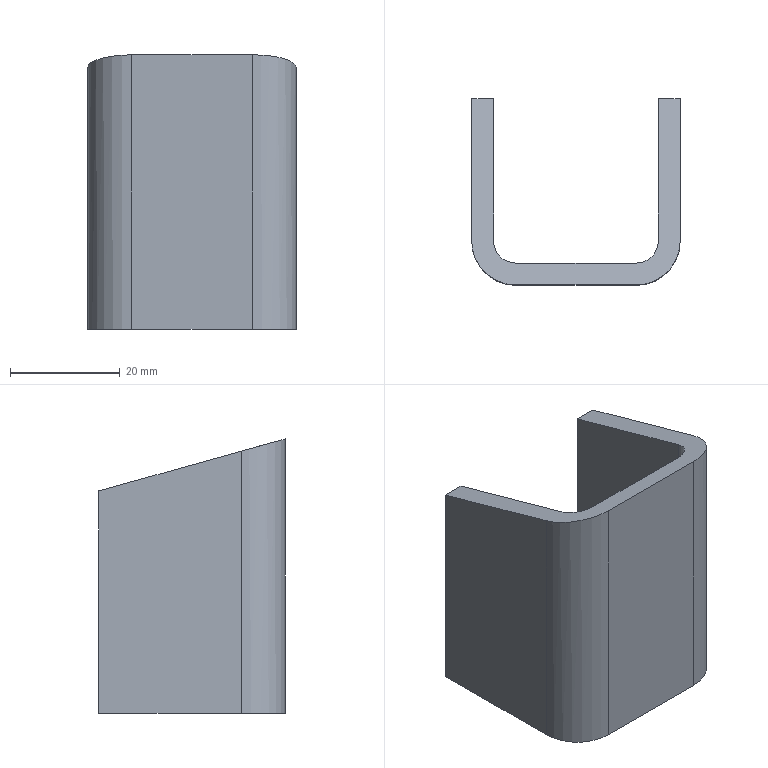Part | STEP file | 18-Reinforcing bent plate 2 | 1 solid | 18 faces | box 38 x 34 x 50 mm | volume 17215 mm3 | plane 14 | cylinder 4 | commonest cylinder face diameters 8 x2 16 x2
STEP:
#1=CARTESIAN_POINT('',(0.,0.,0.));
#2=DIRECTION('',(0.,0.,1.));
#3=DIRECTION('',(1.,0.,0.));
#4=AXIS2_PLACEMENT_3D('',#1,#2,#3);
#5=CARTESIAN_POINT('',(8.,-34.,0.));
#6=VERTEX_POINT('',#5);
#7=CARTESIAN_POINT('',(8.,-30.,0.));
#8=VERTEX_POINT('',#7);
#9=CARTESIAN_POINT('',(8.,-34.,0.));
#10=DIRECTION('',(0.,1.,0.));
#11=VECTOR('',#10,1.);
#12=LINE('',#9,#11);
#13=CARTESIAN_POINT('',(8.,-34.,0.));
#14=DIRECTION('',(0.,0.,-1.));
#15=DIRECTION('',(-1.,0.,0.));
#16=AXIS2_PLACEMENT_3D('',#13,#14,#15);
#17=PLANE('',#16);
#18=CARTESIAN_POINT('',(0.,0.));
#19=DIRECTION('',(0.,1.));
#20=VECTOR('',#19,1.);
#21=LINE('',#18,#20);
#22=(GEOMETRIC_REPRESENTATION_CONTEXT(2)PARAMETRIC_REPRESENTATION_CONTEXT()REPRESENTATION_CONTEXT('',''));
#23=DEFINITIONAL_REPRESENTATION('',(#21),#22);
#24=PCURVE('',#17,#23);
#25=CARTESIAN_POINT('',(4.,-26.,0.));
#26=DIRECTION('',(0.,0.,-1.));
#27=DIRECTION('',(-1.,0.,0.));
#28=AXIS2_PLACEMENT_3D('',#25,#26,#27);
#29=PLANE('',#28);
#30=CARTESIAN_POINT('',(-4.,-8.));
#31=DIRECTION('',(0.,1.));
#32=VECTOR('',#31,1.);
#33=LINE('',#30,#32);
#34=(GEOMETRIC_REPRESENTATION_CONTEXT(2)PARAMETRIC_REPRESENTATION_CONTEXT()REPRESENTATION_CONTEXT('',''));
#35=DEFINITIONAL_REPRESENTATION('',(#33),#34);
#36=PCURVE('',#29,#35);
#37=SURFACE_CURVE('',#12,(#24,#36),.PCURVE_S1.);
#38=EDGE_CURVE('',#6,#8,#37,.T.);
#39=ORIENTED_EDGE('',*,*,#38,.F.);
#40=CARTESIAN_POINT('',(0.,-26.,0.));
#41=VERTEX_POINT('',#40);
#42=CARTESIAN_POINT('',(8.,-26.,0.));
#43=DIRECTION('',(0.,0.,1.));
#44=DIRECTION('',(-1.,0.,0.));
#45=AXIS2_PLACEMENT_3D('',#42,#43,#44);
#46=CIRCLE('',#45,8.);
#47=CARTESIAN_POINT('',(8.,8.));
#48=CARTESIAN_POINT('',(8.,-5.856));
#49=CARTESIAN_POINT('',(-4.,1.072));
#50=CARTESIAN_POINT('',(-16.,8.));
#51=CARTESIAN_POINT('',(-4.,14.928));
#52=CARTESIAN_POINT('',(8.,21.856));
#53=CARTESIAN_POINT('',(8.,8.));
#54=(BOUNDED_CURVE()B_SPLINE_CURVE(2,(#47,#48,#49,#50,#51,#52,#53),.UNSPECIFIED.,.T.,.F.)B_SPLINE_CURVE_WITH_KNOTS((1,2,2,2,2,1),(-2.094,0.,2.094,4.189,6.283,8.378),.UNSPECIFIED.)CURVE()GEOMETRIC_REPRESENTATION_ITEM()RATIONAL_B_SPLINE_CURVE((1.,0.5,1.,0.5,1.,0.5,1.))REPRESENTATION_ITEM(''));
#55=(GEOMETRIC_REPRESENTATION_CONTEXT(2)PARAMETRIC_REPRESENTATION_CONTEXT()REPRESENTATION_CONTEXT('',''));
#56=DEFINITIONAL_REPRESENTATION('',(#54),#55);
#57=PCURVE('',#17,#56);
#58=CARTESIAN_POINT('',(8.,-26.,50.));
#59=DIRECTION('',(0.,0.,-1.));
#60=DIRECTION('',(-1.,0.,0.));
#61=AXIS2_PLACEMENT_3D('',#58,#59,#60);
#62=CYLINDRICAL_SURFACE('',#61,8.);
#63=CARTESIAN_POINT('',(6.283,50.));
#64=DIRECTION('',(-1.,0.));
#65=VECTOR('',#64,1.);
#66=LINE('',#63,#65);
#67=(GEOMETRIC_REPRESENTATION_CONTEXT(2)PARAMETRIC_REPRESENTATION_CONTEXT()REPRESENTATION_CONTEXT('',''));
#68=DEFINITIONAL_REPRESENTATION('',(#66),#67);
#69=PCURVE('',#62,#68);
#70=SURFACE_CURVE('',#46,(#57,#69),.PCURVE_S1.);
#71=EDGE_CURVE('',#41,#6,#70,.T.);
#72=ORIENTED_EDGE('',*,*,#71,.F.);
#73=CARTESIAN_POINT('',(4.,-26.,0.));
#74=VERTEX_POINT('',#73);
#75=CARTESIAN_POINT('',(4.,-26.,0.));
#76=DIRECTION('',(-1.,0.,0.));
#77=VECTOR('',#76,1.);
#78=LINE('',#75,#77);
#79=CARTESIAN_POINT('',(4.,8.));
#80=DIRECTION('',(1.,0.));
#81=VECTOR('',#80,1.);
#82=LINE('',#79,#81);
#83=(GEOMETRIC_REPRESENTATION_CONTEXT(2)PARAMETRIC_REPRESENTATION_CONTEXT()REPRESENTATION_CONTEXT('',''));
#84=DEFINITIONAL_REPRESENTATION('',(#82),#83);
#85=PCURVE('',#17,#84);
#86=CARTESIAN_POINT('',(30.,-26.,0.));
#87=DIRECTION('',(0.,0.,1.));
#88=DIRECTION('',(1.,0.,0.));
#89=AXIS2_PLACEMENT_3D('',#86,#87,#88);
#90=PLANE('',#89);
#91=CARTESIAN_POINT('',(-26.,0.));
#92=DIRECTION('',(-1.,0.));
#93=VECTOR('',#92,1.);
#94=LINE('',#91,#93);
#95=(GEOMETRIC_REPRESENTATION_CONTEXT(2)PARAMETRIC_REPRESENTATION_CONTEXT()REPRESENTATION_CONTEXT('',''));
#96=DEFINITIONAL_REPRESENTATION('',(#94),#95);
#97=PCURVE('',#90,#96);
#98=SURFACE_CURVE('',#78,(#85,#97),.PCURVE_S1.);
#99=EDGE_CURVE('',#74,#41,#98,.T.);
#100=ORIENTED_EDGE('',*,*,#99,.F.);
#101=CARTESIAN_POINT('',(8.,-26.,0.));
#102=DIRECTION('',(0.,0.,1.));
#103=DIRECTION('',(1.,0.,0.));
#104=AXIS2_PLACEMENT_3D('',#101,#102,#103);
#105=CIRCLE('',#104,4.);
#106=CARTESIAN_POINT('',(-4.,8.));
#107=CARTESIAN_POINT('',(-4.,14.928));
#108=CARTESIAN_POINT('',(2.,11.464));
#109=CARTESIAN_POINT('',(8.,8.));
#110=CARTESIAN_POINT('',(2.,4.536));
#111=CARTESIAN_POINT('',(-4.,1.072));
#112=CARTESIAN_POINT('',(-4.,8.));
#113=(BOUNDED_CURVE()B_SPLINE_CURVE(2,(#106,#107,#108,#109,#110,#111,#112),.UNSPECIFIED.,.T.,.F.)B_SPLINE_CURVE_WITH_KNOTS((1,2,2,2,2,1),(-2.094,0.,2.094,4.189,6.283,8.378),.UNSPECIFIED.)CURVE()GEOMETRIC_REPRESENTATION_ITEM()RATIONAL_B_SPLINE_CURVE((1.,0.5,1.,0.5,1.,0.5,1.))REPRESENTATION_ITEM(''));
#114=(GEOMETRIC_REPRESENTATION_CONTEXT(2)PARAMETRIC_REPRESENTATION_CONTEXT()REPRESENTATION_CONTEXT('',''));
#115=DEFINITIONAL_REPRESENTATION('',(#113),#114);
#116=PCURVE('',#17,#115);
#117=CARTESIAN_POINT('',(8.,-26.,50.));
#118=DIRECTION('',(0.,0.,-1.));
#119=DIRECTION('',(-1.,0.,0.));
#120=AXIS2_PLACEMENT_3D('',#117,#118,#119);
#121=CYLINDRICAL_SURFACE('',#120,4.);
#122=CARTESIAN_POINT('',(9.425,50.));
#123=DIRECTION('',(-1.,0.));
#124=VECTOR('',#123,1.);
#125=LINE('',#122,#124);
#126=(GEOMETRIC_REPRESENTATION_CONTEXT(2)PARAMETRIC_REPRESENTATION_CONTEXT()REPRESENTATION_CONTEXT('',''));
#127=DEFINITIONAL_REPRESENTATION('',(#125),#126);
#128=PCURVE('',#121,#127);
#129=SURFACE_CURVE('',#105,(#116,#128),.PCURVE_S1.);
#130=EDGE_CURVE('',#74,#8,#129,.T.);
#131=ORIENTED_EDGE('',*,*,#130,.T.);
#132=EDGE_LOOP('',(#39,#72,#100,#131));
#133=FACE_BOUND('',#132,.T.);
#134=ADVANCED_FACE('',(#133),#17,.T.);
#135=CARTESIAN_POINT('',(30.,-34.,0.));
#136=VERTEX_POINT('',#135);
#137=CARTESIAN_POINT('',(0.,-34.,0.));
#138=DIRECTION('',(1.,0.,0.));
#139=VECTOR('',#138,1.);
#140=LINE('',#137,#139);
#141=CARTESIAN_POINT('',(4.,-8.));
#142=DIRECTION('',(-1.,0.));
#143=VECTOR('',#142,1.);
#144=LINE('',#141,#143);
#145=(GEOMETRIC_REPRESENTATION_CONTEXT(2)PARAMETRIC_REPRESENTATION_CONTEXT()REPRESENTATION_CONTEXT('',''));
#146=DEFINITIONAL_REPRESENTATION('',(#144),#145);
#147=PCURVE('',#29,#146);
#148=CARTESIAN_POINT('',(0.,-34.,50.));
#149=DIRECTION('',(0.,1.,0.));
#150=DIRECTION('',(0.,0.,1.));
#151=AXIS2_PLACEMENT_3D('',#148,#149,#150);
#152=PLANE('',#151);
#153=CARTESIAN_POINT('',(-50.,0.));
#154=DIRECTION('',(0.,1.));
#155=VECTOR('',#154,1.);
#156=LINE('',#153,#155);
#157=(GEOMETRIC_REPRESENTATION_CONTEXT(2)PARAMETRIC_REPRESENTATION_CONTEXT()REPRESENTATION_CONTEXT('',''));
#158=DEFINITIONAL_REPRESENTATION('',(#156),#157);
#159=PCURVE('',#152,#158);
#160=SURFACE_CURVE('',#140,(#147,#159),.PCURVE_S1.);
#161=EDGE_CURVE('',#6,#136,#160,.T.);
#162=ORIENTED_EDGE('',*,*,#161,.F.);
#163=ORIENTED_EDGE('',*,*,#38,.T.);
#164=CARTESIAN_POINT('',(30.,-30.,0.));
#165=VERTEX_POINT('',#164);
#166=CARTESIAN_POINT('',(0.,-30.,0.));
#167=DIRECTION('',(1.,0.,0.));
#168=VECTOR('',#167,1.);
#169=LINE('',#166,#168);
#170=CARTESIAN_POINT('',(4.,-4.));
#171=DIRECTION('',(-1.,0.));
#172=VECTOR('',#171,1.);
#173=LINE('',#170,#172);
#174=(GEOMETRIC_REPRESENTATION_CONTEXT(2)PARAMETRIC_REPRESENTATION_CONTEXT()REPRESENTATION_CONTEXT('',''));
#175=DEFINITIONAL_REPRESENTATION('',(#173),#174);
#176=PCURVE('',#29,#175);
#177=CARTESIAN_POINT('',(0.,-30.,50.));
#178=DIRECTION('',(0.,1.,0.));
#179=DIRECTION('',(0.,0.,1.));
#180=AXIS2_PLACEMENT_3D('',#177,#178,#179);
#181=PLANE('',#180);
#182=CARTESIAN_POINT('',(-50.,0.));
#183=DIRECTION('',(0.,1.));
#184=VECTOR('',#183,1.);
#185=LINE('',#182,#184);
#186=(GEOMETRIC_REPRESENTATION_CONTEXT(2)PARAMETRIC_REPRESENTATION_CONTEXT()REPRESENTATION_CONTEXT('',''));
#187=DEFINITIONAL_REPRESENTATION('',(#185),#186);
#188=PCURVE('',#181,#187);
#189=SURFACE_CURVE('',#169,(#176,#188),.PCURVE_S1.);
#190=EDGE_CURVE('',#8,#165,#189,.T.);
#191=ORIENTED_EDGE('',*,*,#190,.T.);
#192=CARTESIAN_POINT('',(30.,-30.,0.));
#193=DIRECTION('',(0.,-1.,0.));
#194=VECTOR('',#193,1.);
#195=LINE('',#192,#194);
#196=CARTESIAN_POINT('',(-26.,-4.));
#197=DIRECTION('',(0.,-1.));
#198=VECTOR('',#197,1.);
#199=LINE('',#196,#198);
#200=(GEOMETRIC_REPRESENTATION_CONTEXT(2)PARAMETRIC_REPRESENTATION_CONTEXT()REPRESENTATION_CONTEXT('',''));
#201=DEFINITIONAL_REPRESENTATION('',(#199),#200);
#202=PCURVE('',#29,#201);
#203=CARTESIAN_POINT('',(38.,-26.,0.));
#204=DIRECTION('',(0.,0.,-1.));
#205=DIRECTION('',(-1.,0.,0.));
#206=AXIS2_PLACEMENT_3D('',#203,#204,#205);
#207=PLANE('',#206);
#208=CARTESIAN_POINT('',(8.,-4.));
#209=DIRECTION('',(0.,-1.));
#210=VECTOR('',#209,1.);
#211=LINE('',#208,#210);
#212=(GEOMETRIC_REPRESENTATION_CONTEXT(2)PARAMETRIC_REPRESENTATION_CONTEXT()REPRESENTATION_CONTEXT('',''));
#213=DEFINITIONAL_REPRESENTATION('',(#211),#212);
#214=PCURVE('',#207,#213);
#215=SURFACE_CURVE('',#195,(#202,#214),.PCURVE_S1.);
#216=EDGE_CURVE('',#165,#136,#215,.T.);
#217=ORIENTED_EDGE('',*,*,#216,.T.);
#218=EDGE_LOOP('',(#162,#163,#191,#217));
#219=FACE_BOUND('',#218,.T.);
#220=ADVANCED_FACE('',(#219),#29,.T.);
#221=CARTESIAN_POINT('',(38.,-26.,0.));
#222=VERTEX_POINT('',#221);
#223=CARTESIAN_POINT('',(34.,-26.,0.));
#224=VERTEX_POINT('',#223);
#225=CARTESIAN_POINT('',(38.,-26.,0.));
#226=DIRECTION('',(-1.,0.,0.));
#227=VECTOR('',#226,1.);
#228=LINE('',#225,#227);
#229=CARTESIAN_POINT('',(0.,0.));
#230=DIRECTION('',(1.,0.));
#231=VECTOR('',#230,1.);
#232=LINE('',#229,#231);
#233=(GEOMETRIC_REPRESENTATION_CONTEXT(2)PARAMETRIC_REPRESENTATION_CONTEXT()REPRESENTATION_CONTEXT('',''));
#234=DEFINITIONAL_REPRESENTATION('',(#232),#233);
#235=PCURVE('',#207,#234);
#236=CARTESIAN_POINT('',(30.,-30.,0.));
#237=DIRECTION('',(0.,0.,-1.));
#238=DIRECTION('',(-1.,0.,0.));
#239=AXIS2_PLACEMENT_3D('',#236,#237,#238);
#240=PLANE('',#239);
#241=CARTESIAN_POINT('',(-8.,4.));
#242=DIRECTION('',(1.,0.));
#243=VECTOR('',#242,1.);
#244=LINE('',#241,#243);
#245=(GEOMETRIC_REPRESENTATION_CONTEXT(2)PARAMETRIC_REPRESENTATION_CONTEXT()REPRESENTATION_CONTEXT('',''));
#246=DEFINITIONAL_REPRESENTATION('',(#244),#245);
#247=PCURVE('',#240,#246);
#248=SURFACE_CURVE('',#228,(#235,#247),.PCURVE_S1.);
#249=EDGE_CURVE('',#222,#224,#248,.T.);
#250=ORIENTED_EDGE('',*,*,#249,.F.);
#251=CARTESIAN_POINT('',(30.,-26.,0.));
#252=DIRECTION('',(0.,0.,1.));
#253=DIRECTION('',(-1.,0.,0.));
#254=AXIS2_PLACEMENT_3D('',#251,#252,#253);
#255=CIRCLE('',#254,8.);
#256=CARTESIAN_POINT('',(16.,0.));
#257=CARTESIAN_POINT('',(16.,-13.856));
#258=CARTESIAN_POINT('',(4.,-6.928));
#259=CARTESIAN_POINT('',(-8.,0.));
#260=CARTESIAN_POINT('',(4.,6.928));
#261=CARTESIAN_POINT('',(16.,13.856));
#262=CARTESIAN_POINT('',(16.,0.));
#263=(BOUNDED_CURVE()B_SPLINE_CURVE(2,(#256,#257,#258,#259,#260,#261,#262),.UNSPECIFIED.,.T.,.F.)B_SPLINE_CURVE_WITH_KNOTS((1,2,2,2,2,1),(-2.094,0.,2.094,4.189,6.283,8.378),.UNSPECIFIED.)CURVE()GEOMETRIC_REPRESENTATION_ITEM()RATIONAL_B_SPLINE_CURVE((1.,0.5,1.,0.5,1.,0.5,1.))REPRESENTATION_ITEM(''));
#264=(GEOMETRIC_REPRESENTATION_CONTEXT(2)PARAMETRIC_REPRESENTATION_CONTEXT()REPRESENTATION_CONTEXT('',''));
#265=DEFINITIONAL_REPRESENTATION('',(#263),#264);
#266=PCURVE('',#207,#265);
#267=CARTESIAN_POINT('',(30.,-26.,50.));
#268=DIRECTION('',(0.,0.,-1.));
#269=DIRECTION('',(-1.,0.,0.));
#270=AXIS2_PLACEMENT_3D('',#267,#268,#269);
#271=CYLINDRICAL_SURFACE('',#270,8.);
#272=CARTESIAN_POINT('',(6.283,50.));
#273=DIRECTION('',(-1.,0.));
#274=VECTOR('',#273,1.);
#275=LINE('',#272,#274);
#276=(GEOMETRIC_REPRESENTATION_CONTEXT(2)PARAMETRIC_REPRESENTATION_CONTEXT()REPRESENTATION_CONTEXT('',''));
#277=DEFINITIONAL_REPRESENTATION('',(#275),#276);
#278=PCURVE('',#271,#277);
#279=SURFACE_CURVE('',#255,(#266,#278),.PCURVE_S1.);
#280=EDGE_CURVE('',#136,#222,#279,.T.);
#281=ORIENTED_EDGE('',*,*,#280,.F.);
#282=ORIENTED_EDGE('',*,*,#216,.F.);
#283=CARTESIAN_POINT('',(30.,-26.,0.));
#284=DIRECTION('',(0.,0.,1.));
#285=DIRECTION('',(1.,0.,0.));
#286=AXIS2_PLACEMENT_3D('',#283,#284,#285);
#287=CIRCLE('',#286,4.);
#288=CARTESIAN_POINT('',(4.,0.));
#289=CARTESIAN_POINT('',(4.,6.928));
#290=CARTESIAN_POINT('',(10.,3.464));
#291=CARTESIAN_POINT('',(16.,0.));
#292=CARTESIAN_POINT('',(10.,-3.464));
#293=CARTESIAN_POINT('',(4.,-6.928));
#294=CARTESIAN_POINT('',(4.,0.));
#295=(BOUNDED_CURVE()B_SPLINE_CURVE(2,(#288,#289,#290,#291,#292,#293,#294),.UNSPECIFIED.,.T.,.F.)B_SPLINE_CURVE_WITH_KNOTS((1,2,2,2,2,1),(-2.094,0.,2.094,4.189,6.283,8.378),.UNSPECIFIED.)CURVE()GEOMETRIC_REPRESENTATION_ITEM()RATIONAL_B_SPLINE_CURVE((1.,0.5,1.,0.5,1.,0.5,1.))REPRESENTATION_ITEM(''));
#296=(GEOMETRIC_REPRESENTATION_CONTEXT(2)PARAMETRIC_REPRESENTATION_CONTEXT()REPRESENTATION_CONTEXT('',''));
#297=DEFINITIONAL_REPRESENTATION('',(#295),#296);
#298=PCURVE('',#207,#297);
#299=CARTESIAN_POINT('',(30.,-26.,50.));
#300=DIRECTION('',(0.,0.,-1.));
#301=DIRECTION('',(-1.,0.,0.));
#302=AXIS2_PLACEMENT_3D('',#299,#300,#301);
#303=CYLINDRICAL_SURFACE('',#302,4.);
#304=CARTESIAN_POINT('',(9.425,50.));
#305=DIRECTION('',(-1.,0.));
#306=VECTOR('',#305,1.);
#307=LINE('',#304,#306);
#308=(GEOMETRIC_REPRESENTATION_CONTEXT(2)PARAMETRIC_REPRESENTATION_CONTEXT()REPRESENTATION_CONTEXT('',''));
#309=DEFINITIONAL_REPRESENTATION('',(#307),#308);
#310=PCURVE('',#303,#309);
#311=SURFACE_CURVE('',#287,(#298,#310),.PCURVE_S1.);
#312=EDGE_CURVE('',#165,#224,#311,.T.);
#313=ORIENTED_EDGE('',*,*,#312,.T.);
#314=EDGE_LOOP('',(#250,#281,#282,#313));
#315=FACE_BOUND('',#314,.T.);
#316=ADVANCED_FACE('',(#315),#207,.T.);
#317=CARTESIAN_POINT('',(38.,0.,0.));
#318=VERTEX_POINT('',#317);
#319=CARTESIAN_POINT('',(38.,-34.,0.));
#320=DIRECTION('',(0.,1.,0.));
#321=VECTOR('',#320,1.);
#322=LINE('',#319,#321);
#323=CARTESIAN_POINT('',(-8.,-4.));
#324=DIRECTION('',(0.,1.));
#325=VECTOR('',#324,1.);
#326=LINE('',#323,#325);
#327=(GEOMETRIC_REPRESENTATION_CONTEXT(2)PARAMETRIC_REPRESENTATION_CONTEXT()REPRESENTATION_CONTEXT('',''));
#328=DEFINITIONAL_REPRESENTATION('',(#326),#327);
#329=PCURVE('',#240,#328);
#330=CARTESIAN_POINT('',(38.,-34.,50.));
#331=DIRECTION('',(-1.,0.,0.));
#332=DIRECTION('',(0.,0.,1.));
#333=AXIS2_PLACEMENT_3D('',#330,#331,#332);
#334=PLANE('',#333);
#335=CARTESIAN_POINT('',(-50.,0.));
#336=DIRECTION('',(0.,1.));
#337=VECTOR('',#336,1.);
#338=LINE('',#335,#337);
#339=(GEOMETRIC_REPRESENTATION_CONTEXT(2)PARAMETRIC_REPRESENTATION_CONTEXT()REPRESENTATION_CONTEXT('',''));
#340=DEFINITIONAL_REPRESENTATION('',(#338),#339);
#341=PCURVE('',#334,#340);
#342=SURFACE_CURVE('',#322,(#329,#341),.PCURVE_S1.);
#343=EDGE_CURVE('',#222,#318,#342,.T.);
#344=ORIENTED_EDGE('',*,*,#343,.F.);
#345=ORIENTED_EDGE('',*,*,#249,.T.);
#346=CARTESIAN_POINT('',(34.,0.,0.));
#347=VERTEX_POINT('',#346);
#348=CARTESIAN_POINT('',(34.,-34.,0.));
#349=DIRECTION('',(0.,1.,0.));
#350=VECTOR('',#349,1.);
#351=LINE('',#348,#350);
#352=CARTESIAN_POINT('',(-4.,-4.));
#353=DIRECTION('',(0.,1.));
#354=VECTOR('',#353,1.);
#355=LINE('',#352,#354);
#356=(GEOMETRIC_REPRESENTATION_CONTEXT(2)PARAMETRIC_REPRESENTATION_CONTEXT()REPRESENTATION_CONTEXT('',''));
#357=DEFINITIONAL_REPRESENTATION('',(#355),#356);
#358=PCURVE('',#240,#357);
#359=CARTESIAN_POINT('',(34.,-34.,50.));
#360=DIRECTION('',(-1.,0.,0.));
#361=DIRECTION('',(0.,0.,1.));
#362=AXIS2_PLACEMENT_3D('',#359,#360,#361);
#363=PLANE('',#362);
#364=CARTESIAN_POINT('',(-50.,0.));
#365=DIRECTION('',(0.,1.));
#366=VECTOR('',#365,1.);
#367=LINE('',#364,#366);
#368=(GEOMETRIC_REPRESENTATION_CONTEXT(2)PARAMETRIC_REPRESENTATION_CONTEXT()REPRESENTATION_CONTEXT('',''));
#369=DEFINITIONAL_REPRESENTATION('',(#367),#368);
#370=PCURVE('',#363,#369);
#371=SURFACE_CURVE('',#351,(#358,#370),.PCURVE_S1.);
#372=EDGE_CURVE('',#224,#347,#371,.T.);
#373=ORIENTED_EDGE('',*,*,#372,.T.);
#374=CARTESIAN_POINT('',(34.,0.,0.));
#375=DIRECTION('',(1.,0.,0.));
#376=VECTOR('',#375,1.);
#377=LINE('',#374,#376);
#378=CARTESIAN_POINT('',(-4.,30.));
#379=DIRECTION('',(-1.,0.));
#380=VECTOR('',#379,1.);
#381=LINE('',#378,#380);
#382=(GEOMETRIC_REPRESENTATION_CONTEXT(2)PARAMETRIC_REPRESENTATION_CONTEXT()REPRESENTATION_CONTEXT('',''));
#383=DEFINITIONAL_REPRESENTATION('',(#381),#382);
#384=PCURVE('',#240,#383);
#385=CARTESIAN_POINT('',(34.,0.,50.));
#386=DIRECTION('',(0.,1.,0.));
#387=DIRECTION('',(0.,0.,1.));
#388=AXIS2_PLACEMENT_3D('',#385,#386,#387);
#389=PLANE('',#388);
#390=CARTESIAN_POINT('',(-50.,0.));
#391=DIRECTION('',(0.,1.));
#392=VECTOR('',#391,1.);
#393=LINE('',#390,#392);
#394=(GEOMETRIC_REPRESENTATION_CONTEXT(2)PARAMETRIC_REPRESENTATION_CONTEXT()REPRESENTATION_CONTEXT('',''));
#395=DEFINITIONAL_REPRESENTATION('',(#393),#394);
#396=PCURVE('',#389,#395);
#397=SURFACE_CURVE('',#377,(#384,#396),.PCURVE_S1.);
#398=EDGE_CURVE('',#347,#318,#397,.T.);
#399=ORIENTED_EDGE('',*,*,#398,.T.);
#400=EDGE_LOOP('',(#344,#345,#373,#399));
#401=FACE_BOUND('',#400,.T.);
#402=ADVANCED_FACE('',(#401),#240,.T.);
#403=CARTESIAN_POINT('',(38.,0.,40.5));
#404=VERTEX_POINT('',#403);
#405=CARTESIAN_POINT('',(38.,0.,50.));
#406=DIRECTION('',(0.,0.,-1.));
#407=VECTOR('',#406,1.);
#408=LINE('',#405,#407);
#409=CARTESIAN_POINT('',(0.,34.));
#410=DIRECTION('',(-1.,0.));
#411=VECTOR('',#410,1.);
#412=LINE('',#409,#411);
#413=(GEOMETRIC_REPRESENTATION_CONTEXT(2)PARAMETRIC_REPRESENTATION_CONTEXT()REPRESENTATION_CONTEXT('',''));
#414=DEFINITIONAL_REPRESENTATION('',(#412),#413);
#415=PCURVE('',#334,#414);
#416=CARTESIAN_POINT('',(0.,4.));
#417=DIRECTION('',(-1.,0.));
#418=VECTOR('',#417,1.);
#419=LINE('',#416,#418);
#420=(GEOMETRIC_REPRESENTATION_CONTEXT(2)PARAMETRIC_REPRESENTATION_CONTEXT()REPRESENTATION_CONTEXT('',''));
#421=DEFINITIONAL_REPRESENTATION('',(#419),#420);
#422=PCURVE('',#389,#421);
#423=SURFACE_CURVE('',#408,(#415,#422),.PCURVE_S1.);
#424=EDGE_CURVE('',#404,#318,#423,.T.);
#425=ORIENTED_EDGE('',*,*,#424,.F.);
#426=CARTESIAN_POINT('',(38.,-26.,47.765));
#427=VERTEX_POINT('',#426);
#428=CARTESIAN_POINT('',(38.,-34.,50.));
#429=DIRECTION('',(0.,-0.9631,0.2691));
#430=VECTOR('',#429,1.);
#431=LINE('',#428,#430);
#432=CARTESIAN_POINT('',(0.,0.));
#433=DIRECTION('',(0.2691,-0.9631));
#434=VECTOR('',#433,1.);
#435=LINE('',#432,#434);
#436=(GEOMETRIC_REPRESENTATION_CONTEXT(2)PARAMETRIC_REPRESENTATION_CONTEXT()REPRESENTATION_CONTEXT('',''));
#437=DEFINITIONAL_REPRESENTATION('',(#435),#436);
#438=PCURVE('',#334,#437);
#439=CARTESIAN_POINT('',(38.,-34.,50.));
#440=DIRECTION('',(0.,-0.2691,-0.9631));
#441=DIRECTION('',(0.,0.9631,-0.2691));
#442=AXIS2_PLACEMENT_3D('',#439,#440,#441);
#443=PLANE('',#442);
#444=CARTESIAN_POINT('',(0.,0.));
#445=DIRECTION('',(-1.,0.));
#446=VECTOR('',#445,1.);
#447=LINE('',#444,#446);
#448=(GEOMETRIC_REPRESENTATION_CONTEXT(2)PARAMETRIC_REPRESENTATION_CONTEXT()REPRESENTATION_CONTEXT('',''));
#449=DEFINITIONAL_REPRESENTATION('',(#447),#448);
#450=PCURVE('',#443,#449);
#451=SURFACE_CURVE('',#431,(#438,#450),.PCURVE_S1.);
#452=EDGE_CURVE('',#404,#427,#451,.T.);
#453=ORIENTED_EDGE('',*,*,#452,.T.);
#454=CARTESIAN_POINT('',(38.,-26.,50.));
#455=DIRECTION('',(0.,0.,-1.));
#456=VECTOR('',#455,1.);
#457=LINE('',#454,#456);
#458=CARTESIAN_POINT('',(0.,8.));
#459=DIRECTION('',(-1.,0.));
#460=VECTOR('',#459,1.);
#461=LINE('',#458,#460);
#462=(GEOMETRIC_REPRESENTATION_CONTEXT(2)PARAMETRIC_REPRESENTATION_CONTEXT()REPRESENTATION_CONTEXT('',''));
#463=DEFINITIONAL_REPRESENTATION('',(#461),#462);
#464=PCURVE('',#334,#463);
#465=CARTESIAN_POINT('',(3.142,0.));
#466=DIRECTION('',(0.,1.));
#467=VECTOR('',#466,1.);
#468=LINE('',#465,#467);
#469=(GEOMETRIC_REPRESENTATION_CONTEXT(2)PARAMETRIC_REPRESENTATION_CONTEXT()REPRESENTATION_CONTEXT('',''));
#470=DEFINITIONAL_REPRESENTATION('',(#468),#469);
#471=PCURVE('',#271,#470);
#472=SURFACE_CURVE('',#457,(#464,#471),.PCURVE_S1.);
#473=EDGE_CURVE('',#427,#222,#472,.T.);
#474=ORIENTED_EDGE('',*,*,#473,.T.);
#475=ORIENTED_EDGE('',*,*,#343,.T.);
#476=EDGE_LOOP('',(#425,#453,#474,#475));
#477=FACE_BOUND('',#476,.T.);
#478=ADVANCED_FACE('',(#477),#334,.F.);
#479=CARTESIAN_POINT('',(34.,0.,40.5));
#480=VERTEX_POINT('',#479);
#481=CARTESIAN_POINT('',(38.,0.,40.5));
#482=DIRECTION('',(-1.,0.,0.));
#483=VECTOR('',#482,1.);
#484=LINE('',#481,#483);
#485=CARTESIAN_POINT('',(-9.5,4.));
#486=DIRECTION('',(0.,-1.));
#487=VECTOR('',#486,1.);
#488=LINE('',#485,#487);
#489=(GEOMETRIC_REPRESENTATION_CONTEXT(2)PARAMETRIC_REPRESENTATION_CONTEXT()REPRESENTATION_CONTEXT('',''));
#490=DEFINITIONAL_REPRESENTATION('',(#488),#489);
#491=PCURVE('',#389,#490);
#492=CARTESIAN_POINT('',(35.302,0.));
#493=DIRECTION('',(0.,-1.));
#494=VECTOR('',#493,1.);
#495=LINE('',#492,#494);
#496=(GEOMETRIC_REPRESENTATION_CONTEXT(2)PARAMETRIC_REPRESENTATION_CONTEXT()REPRESENTATION_CONTEXT('',''));
#497=DEFINITIONAL_REPRESENTATION('',(#495),#496);
#498=PCURVE('',#443,#497);
#499=SURFACE_CURVE('',#484,(#491,#498),.PCURVE_S1.);
#500=EDGE_CURVE('',#404,#480,#499,.T.);
#501=ORIENTED_EDGE('',*,*,#500,.F.);
#502=ORIENTED_EDGE('',*,*,#424,.T.);
#503=ORIENTED_EDGE('',*,*,#398,.F.);
#504=CARTESIAN_POINT('',(34.,0.,50.));
#505=DIRECTION('',(0.,0.,-1.));
#506=VECTOR('',#505,1.);
#507=LINE('',#504,#506);
#508=CARTESIAN_POINT('',(0.,0.));
#509=DIRECTION('',(-1.,0.));
#510=VECTOR('',#509,1.);
#511=LINE('',#508,#510);
#512=(GEOMETRIC_REPRESENTATION_CONTEXT(2)PARAMETRIC_REPRESENTATION_CONTEXT()REPRESENTATION_CONTEXT('',''));
#513=DEFINITIONAL_REPRESENTATION('',(#511),#512);
#514=PCURVE('',#389,#513);
#515=CARTESIAN_POINT('',(0.,34.));
#516=DIRECTION('',(-1.,0.));
#517=VECTOR('',#516,1.);
#518=LINE('',#515,#517);
#519=(GEOMETRIC_REPRESENTATION_CONTEXT(2)PARAMETRIC_REPRESENTATION_CONTEXT()REPRESENTATION_CONTEXT('',''));
#520=DEFINITIONAL_REPRESENTATION('',(#518),#519);
#521=PCURVE('',#363,#520);
#522=SURFACE_CURVE('',#507,(#514,#521),.PCURVE_S1.);
#523=EDGE_CURVE('',#480,#347,#522,.T.);
#524=ORIENTED_EDGE('',*,*,#523,.F.);
#525=EDGE_LOOP('',(#501,#502,#503,#524));
#526=FACE_BOUND('',#525,.T.);
#527=ADVANCED_FACE('',(#526),#389,.T.);
#528=CARTESIAN_POINT('',(34.,-26.,47.765));
#529=VERTEX_POINT('',#528);
#530=CARTESIAN_POINT('',(34.,-34.,50.));
#531=DIRECTION('',(0.,-0.9631,0.2691));
#532=VECTOR('',#531,1.);
#533=LINE('',#530,#532);
#534=CARTESIAN_POINT('',(0.,0.));
#535=DIRECTION('',(0.2691,-0.9631));
#536=VECTOR('',#535,1.);
#537=LINE('',#534,#536);
#538=(GEOMETRIC_REPRESENTATION_CONTEXT(2)PARAMETRIC_REPRESENTATION_CONTEXT()REPRESENTATION_CONTEXT('',''));
#539=DEFINITIONAL_REPRESENTATION('',(#537),#538);
#540=PCURVE('',#363,#539);
#541=CARTESIAN_POINT('',(0.,-4.));
#542=DIRECTION('',(-1.,0.));
#543=VECTOR('',#542,1.);
#544=LINE('',#541,#543);
#545=(GEOMETRIC_REPRESENTATION_CONTEXT(2)PARAMETRIC_REPRESENTATION_CONTEXT()REPRESENTATION_CONTEXT('',''));
#546=DEFINITIONAL_REPRESENTATION('',(#544),#545);
#547=PCURVE('',#443,#546);
#548=SURFACE_CURVE('',#533,(#540,#547),.PCURVE_S1.);
#549=EDGE_CURVE('',#480,#529,#548,.T.);
#550=ORIENTED_EDGE('',*,*,#549,.F.);
#551=ORIENTED_EDGE('',*,*,#523,.T.);
#552=ORIENTED_EDGE('',*,*,#372,.F.);
#553=CARTESIAN_POINT('',(34.,-26.,50.));
#554=DIRECTION('',(0.,0.,-1.));
#555=VECTOR('',#554,1.);
#556=LINE('',#553,#555);
#557=CARTESIAN_POINT('',(0.,8.));
#558=DIRECTION('',(-1.,0.));
#559=VECTOR('',#558,1.);
#560=LINE('',#557,#559);
#561=(GEOMETRIC_REPRESENTATION_CONTEXT(2)PARAMETRIC_REPRESENTATION_CONTEXT()REPRESENTATION_CONTEXT('',''));
#562=DEFINITIONAL_REPRESENTATION('',(#560),#561);
#563=PCURVE('',#363,#562);
#564=CARTESIAN_POINT('',(3.142,0.));
#565=DIRECTION('',(0.,1.));
#566=VECTOR('',#565,1.);
#567=LINE('',#564,#566);
#568=(GEOMETRIC_REPRESENTATION_CONTEXT(2)PARAMETRIC_REPRESENTATION_CONTEXT()REPRESENTATION_CONTEXT('',''));
#569=DEFINITIONAL_REPRESENTATION('',(#567),#568);
#570=PCURVE('',#303,#569);
#571=SURFACE_CURVE('',#556,(#563,#570),.PCURVE_S1.);
#572=EDGE_CURVE('',#529,#224,#571,.T.);
#573=ORIENTED_EDGE('',*,*,#572,.F.);
#574=EDGE_LOOP('',(#550,#551,#552,#573));
#575=FACE_BOUND('',#574,.T.);
#576=ADVANCED_FACE('',(#575),#363,.T.);
#577=CARTESIAN_POINT('',(30.,-30.,48.882));
#578=VERTEX_POINT('',#577);
#579=CARTESIAN_POINT('',(30.,-30.,50.));
#580=DIRECTION('',(0.,0.,-1.));
#581=VECTOR('',#580,1.);
#582=LINE('',#579,#581);
#583=CARTESIAN_POINT('',(4.712,0.));
#584=DIRECTION('',(0.,1.));
#585=VECTOR('',#584,1.);
#586=LINE('',#583,#585);
#587=(GEOMETRIC_REPRESENTATION_CONTEXT(2)PARAMETRIC_REPRESENTATION_CONTEXT()REPRESENTATION_CONTEXT('',''));
#588=DEFINITIONAL_REPRESENTATION('',(#586),#587);
#589=PCURVE('',#303,#588);
#590=CARTESIAN_POINT('',(0.,30.));
#591=DIRECTION('',(-1.,0.));
#592=VECTOR('',#591,1.);
#593=LINE('',#590,#592);
#594=(GEOMETRIC_REPRESENTATION_CONTEXT(2)PARAMETRIC_REPRESENTATION_CONTEXT()REPRESENTATION_CONTEXT('',''));
#595=DEFINITIONAL_REPRESENTATION('',(#593),#594);
#596=PCURVE('',#181,#595);
#597=SURFACE_CURVE('',#582,(#589,#596),.PCURVE_S1.);
#598=EDGE_CURVE('',#578,#165,#597,.T.);
#599=ORIENTED_EDGE('',*,*,#598,.T.);
#600=ORIENTED_EDGE('',*,*,#312,.T.);
#601=ORIENTED_EDGE('',*,*,#572,.F.);
#602=CARTESIAN_POINT('',(34.,-26.,47.765));
#603=CARTESIAN_POINT('',(34.,-28.343,48.419));
#604=CARTESIAN_POINT('',(32.343,-30.,48.882));
#605=CARTESIAN_POINT('',(30.,-30.,48.882));
#606=(BOUNDED_CURVE()B_SPLINE_CURVE(3,(#602,#603,#604,#605),.UNSPECIFIED.,.F.,.F.)B_SPLINE_CURVE_WITH_KNOTS((4,4),(1.571,3.142),.PIECEWISE_BEZIER_KNOTS.)CURVE()GEOMETRIC_REPRESENTATION_ITEM()RATIONAL_B_SPLINE_CURVE((1.,0.8047,0.8047,1.))REPRESENTATION_ITEM(''));
#607=CARTESIAN_POINT('',(3.142,2.235));
#608=CARTESIAN_POINT('',(3.163,2.211));
#609=CARTESIAN_POINT('',(3.206,2.163));
#610=CARTESIAN_POINT('',(3.273,2.088));
#611=CARTESIAN_POINT('',(3.342,2.013));
#612=CARTESIAN_POINT('',(3.411,1.937));
#613=CARTESIAN_POINT('',(3.482,1.861));
#614=CARTESIAN_POINT('',(3.555,1.786));
#615=CARTESIAN_POINT('',(3.628,1.713));
#616=CARTESIAN_POINT('',(3.702,1.641));
#617=CARTESIAN_POINT('',(3.777,1.572));
#618=CARTESIAN_POINT('',(3.852,1.506));
#619=CARTESIAN_POINT('',(3.927,1.444));
#620=CARTESIAN_POINT('',(4.002,1.387));
#621=CARTESIAN_POINT('',(4.077,1.335));
#622=CARTESIAN_POINT('',(4.152,1.288));
#623=CARTESIAN_POINT('',(4.226,1.246));
#624=CARTESIAN_POINT('',(4.299,1.211));
#625=CARTESIAN_POINT('',(4.372,1.181));
#626=CARTESIAN_POINT('',(4.443,1.157));
#627=CARTESIAN_POINT('',(4.512,1.139));
#628=CARTESIAN_POINT('',(4.581,1.126));
#629=CARTESIAN_POINT('',(4.648,1.119));
#630=CARTESIAN_POINT('',(4.691,1.118));
#631=CARTESIAN_POINT('',(4.712,1.118));
#632=B_SPLINE_CURVE_WITH_KNOTS('',3,(#607,#608,#609,#610,#611,#612,#613,#614,#615,#616,#617,#618,#619,#620,#621,#622,#623,#624,#625,#626,#627,#628,#629,#630,#631),.UNSPECIFIED.,.F.,.F.,(4,1,1,1,1,1,1,1,1,1,1,1,1,1,1,1,1,1,1,1,1,1,4),(1.571,1.642,1.714,1.785,1.856,1.928,1.999,2.071,2.142,2.213,2.285,2.356,2.428,2.499,2.57,2.642,2.713,2.785,2.856,2.927,2.999,3.07,3.142),.QUASI_UNIFORM_KNOTS.);
#633=(GEOMETRIC_REPRESENTATION_CONTEXT(2)PARAMETRIC_REPRESENTATION_CONTEXT()REPRESENTATION_CONTEXT('',''));
#634=DEFINITIONAL_REPRESENTATION('',(#632),#633);
#635=PCURVE('',#303,#634);
#636=CARTESIAN_POINT('',(8.306,-4.));
#637=CARTESIAN_POINT('',(5.874,-4.));
#638=CARTESIAN_POINT('',(4.153,-5.657));
#639=CARTESIAN_POINT('',(4.153,-8.));
#640=(BOUNDED_CURVE()B_SPLINE_CURVE(3,(#636,#637,#638,#639),.UNSPECIFIED.,.F.,.F.)B_SPLINE_CURVE_WITH_KNOTS((4,4),(1.571,3.142),.PIECEWISE_BEZIER_KNOTS.)CURVE()GEOMETRIC_REPRESENTATION_ITEM()RATIONAL_B_SPLINE_CURVE((1.,0.8047,0.8047,1.))REPRESENTATION_ITEM(''));
#641=(GEOMETRIC_REPRESENTATION_CONTEXT(2)PARAMETRIC_REPRESENTATION_CONTEXT()REPRESENTATION_CONTEXT('',''));
#642=DEFINITIONAL_REPRESENTATION('',(#640),#641);
#643=PCURVE('',#443,#642);
#644=SURFACE_CURVE('',#606,(#635,#643),.PCURVE_S1.);
#645=EDGE_CURVE('',#529,#578,#644,.T.);
#646=ORIENTED_EDGE('',*,*,#645,.T.);
#647=EDGE_LOOP('',(#599,#600,#601,#646));
#648=FACE_BOUND('',#647,.F.);
#649=ADVANCED_FACE('',(#648),#303,.F.);
#650=CARTESIAN_POINT('',(8.,-30.,48.882));
#651=VERTEX_POINT('',#650);
#652=CARTESIAN_POINT('',(0.,-30.,48.882));
#653=DIRECTION('',(-1.,0.,0.));
#654=VECTOR('',#653,1.);
#655=LINE('',#652,#654);
#656=CARTESIAN_POINT('',(-1.118,0.));
#657=DIRECTION('',(0.,-1.));
#658=VECTOR('',#657,1.);
#659=LINE('',#656,#658);
#660=(GEOMETRIC_REPRESENTATION_CONTEXT(2)PARAMETRIC_REPRESENTATION_CONTEXT()REPRESENTATION_CONTEXT('',''));
#661=DEFINITIONAL_REPRESENTATION('',(#659),#660);
#662=PCURVE('',#181,#661);
#663=CARTESIAN_POINT('',(4.153,-38.));
#664=DIRECTION('',(0.,-1.));
#665=VECTOR('',#664,1.);
#666=LINE('',#663,#665);
#667=(GEOMETRIC_REPRESENTATION_CONTEXT(2)PARAMETRIC_REPRESENTATION_CONTEXT()REPRESENTATION_CONTEXT('',''));
#668=DEFINITIONAL_REPRESENTATION('',(#666),#667);
#669=PCURVE('',#443,#668);
#670=SURFACE_CURVE('',#655,(#662,#669),.PCURVE_S1.);
#671=EDGE_CURVE('',#578,#651,#670,.T.);
#672=ORIENTED_EDGE('',*,*,#671,.F.);
#673=ORIENTED_EDGE('',*,*,#598,.T.);
#674=ORIENTED_EDGE('',*,*,#190,.F.);
#675=CARTESIAN_POINT('',(8.,-30.,50.));
#676=DIRECTION('',(0.,0.,-1.));
#677=VECTOR('',#676,1.);
#678=LINE('',#675,#677);
#679=CARTESIAN_POINT('',(0.,8.));
#680=DIRECTION('',(-1.,0.));
#681=VECTOR('',#680,1.);
#682=LINE('',#679,#681);
#683=(GEOMETRIC_REPRESENTATION_CONTEXT(2)PARAMETRIC_REPRESENTATION_CONTEXT()REPRESENTATION_CONTEXT('',''));
#684=DEFINITIONAL_REPRESENTATION('',(#682),#683);
#685=PCURVE('',#181,#684);
#686=CARTESIAN_POINT('',(4.712,0.));
#687=DIRECTION('',(0.,1.));
#688=VECTOR('',#687,1.);
#689=LINE('',#686,#688);
#690=(GEOMETRIC_REPRESENTATION_CONTEXT(2)PARAMETRIC_REPRESENTATION_CONTEXT()REPRESENTATION_CONTEXT('',''));
#691=DEFINITIONAL_REPRESENTATION('',(#689),#690);
#692=PCURVE('',#121,#691);
#693=SURFACE_CURVE('',#678,(#685,#692),.PCURVE_S1.);
#694=EDGE_CURVE('',#651,#8,#693,.T.);
#695=ORIENTED_EDGE('',*,*,#694,.F.);
#696=EDGE_LOOP('',(#672,#673,#674,#695));
#697=FACE_BOUND('',#696,.T.);
#698=ADVANCED_FACE('',(#697),#181,.T.);
#699=CARTESIAN_POINT('',(4.,-26.,47.765));
#700=VERTEX_POINT('',#699);
#701=CARTESIAN_POINT('',(4.,-26.,50.));
#702=DIRECTION('',(0.,0.,-1.));
#703=VECTOR('',#702,1.);
#704=LINE('',#701,#703);
#705=CARTESIAN_POINT('',(6.283,0.));
#706=DIRECTION('',(0.,1.));
#707=VECTOR('',#706,1.);
#708=LINE('',#705,#707);
#709=(GEOMETRIC_REPRESENTATION_CONTEXT(2)PARAMETRIC_REPRESENTATION_CONTEXT()REPRESENTATION_CONTEXT('',''));
#710=DEFINITIONAL_REPRESENTATION('',(#708),#709);
#711=PCURVE('',#121,#710);
#712=CARTESIAN_POINT('',(4.,0.,50.));
#713=DIRECTION('',(1.,0.,0.));
#714=DIRECTION('',(0.,1.,0.));
#715=AXIS2_PLACEMENT_3D('',#712,#713,#714);
#716=PLANE('',#715);
#717=CARTESIAN_POINT('',(-26.,0.));
#718=DIRECTION('',(0.,-1.));
#719=VECTOR('',#718,1.);
#720=LINE('',#717,#719);
#721=(GEOMETRIC_REPRESENTATION_CONTEXT(2)PARAMETRIC_REPRESENTATION_CONTEXT()REPRESENTATION_CONTEXT('',''));
#722=DEFINITIONAL_REPRESENTATION('',(#720),#721);
#723=PCURVE('',#716,#722);
#724=SURFACE_CURVE('',#704,(#711,#723),.PCURVE_S1.);
#725=EDGE_CURVE('',#700,#74,#724,.T.);
#726=ORIENTED_EDGE('',*,*,#725,.T.);
#727=ORIENTED_EDGE('',*,*,#130,.T.);
#728=ORIENTED_EDGE('',*,*,#694,.F.);
#729=CARTESIAN_POINT('',(8.,-30.,48.882));
#730=CARTESIAN_POINT('',(5.657,-30.,48.882));
#731=CARTESIAN_POINT('',(4.,-28.343,48.419));
#732=CARTESIAN_POINT('',(4.,-26.,47.765));
#733=(BOUNDED_CURVE()B_SPLINE_CURVE(3,(#729,#730,#731,#732),.UNSPECIFIED.,.F.,.F.)B_SPLINE_CURVE_WITH_KNOTS((4,4),(3.142,4.712),.PIECEWISE_BEZIER_KNOTS.)CURVE()GEOMETRIC_REPRESENTATION_ITEM()RATIONAL_B_SPLINE_CURVE((1.,0.8047,0.8047,1.))REPRESENTATION_ITEM(''));
#734=CARTESIAN_POINT('',(4.712,1.118));
#735=CARTESIAN_POINT('',(4.734,1.118));
#736=CARTESIAN_POINT('',(4.777,1.119));
#737=CARTESIAN_POINT('',(4.844,1.126));
#738=CARTESIAN_POINT('',(4.912,1.139));
#739=CARTESIAN_POINT('',(4.982,1.157));
#740=CARTESIAN_POINT('',(5.053,1.181));
#741=CARTESIAN_POINT('',(5.125,1.211));
#742=CARTESIAN_POINT('',(5.199,1.246));
#743=CARTESIAN_POINT('',(5.273,1.288));
#744=CARTESIAN_POINT('',(5.347,1.335));
#745=CARTESIAN_POINT('',(5.422,1.387));
#746=CARTESIAN_POINT('',(5.498,1.444));
#747=CARTESIAN_POINT('',(5.573,1.506));
#748=CARTESIAN_POINT('',(5.648,1.572));
#749=CARTESIAN_POINT('',(5.723,1.641));
#750=CARTESIAN_POINT('',(5.797,1.713));
#751=CARTESIAN_POINT('',(5.87,1.786));
#752=CARTESIAN_POINT('',(5.942,1.861));
#753=CARTESIAN_POINT('',(6.013,1.937));
#754=CARTESIAN_POINT('',(6.083,2.013));
#755=CARTESIAN_POINT('',(6.152,2.088));
#756=CARTESIAN_POINT('',(6.218,2.163));
#757=CARTESIAN_POINT('',(6.262,2.211));
#758=CARTESIAN_POINT('',(6.283,2.235));
#759=B_SPLINE_CURVE_WITH_KNOTS('',3,(#734,#735,#736,#737,#738,#739,#740,#741,#742,#743,#744,#745,#746,#747,#748,#749,#750,#751,#752,#753,#754,#755,#756,#757,#758),.UNSPECIFIED.,.F.,.F.,(4,1,1,1,1,1,1,1,1,1,1,1,1,1,1,1,1,1,1,1,1,1,4),(3.142,3.213,3.284,3.356,3.427,3.499,3.57,3.641,3.713,3.784,3.856,3.927,3.998,4.07,4.141,4.213,4.284,4.355,4.427,4.498,4.57,4.641,4.712),.QUASI_UNIFORM_KNOTS.);
#760=(GEOMETRIC_REPRESENTATION_CONTEXT(2)PARAMETRIC_REPRESENTATION_CONTEXT()REPRESENTATION_CONTEXT('',''));
#761=DEFINITIONAL_REPRESENTATION('',(#759),#760);
#762=PCURVE('',#121,#761);
#763=CARTESIAN_POINT('',(4.153,-30.));
#764=CARTESIAN_POINT('',(4.153,-32.343));
#765=CARTESIAN_POINT('',(5.874,-34.));
#766=CARTESIAN_POINT('',(8.306,-34.));
#767=(BOUNDED_CURVE()B_SPLINE_CURVE(3,(#763,#764,#765,#766),.UNSPECIFIED.,.F.,.F.)B_SPLINE_CURVE_WITH_KNOTS((4,4),(3.142,4.712),.PIECEWISE_BEZIER_KNOTS.)CURVE()GEOMETRIC_REPRESENTATION_ITEM()RATIONAL_B_SPLINE_CURVE((1.,0.8047,0.8047,1.))REPRESENTATION_ITEM(''));
#768=(GEOMETRIC_REPRESENTATION_CONTEXT(2)PARAMETRIC_REPRESENTATION_CONTEXT()REPRESENTATION_CONTEXT('',''));
#769=DEFINITIONAL_REPRESENTATION('',(#767),#768);
#770=PCURVE('',#443,#769);
#771=SURFACE_CURVE('',#733,(#762,#770),.PCURVE_S1.);
#772=EDGE_CURVE('',#651,#700,#771,.T.);
#773=ORIENTED_EDGE('',*,*,#772,.T.);
#774=EDGE_LOOP('',(#726,#727,#728,#773));
#775=FACE_BOUND('',#774,.F.);
#776=ADVANCED_FACE('',(#775),#121,.F.);
#777=CARTESIAN_POINT('',(4.,0.,40.5));
#778=VERTEX_POINT('',#777);
#779=CARTESIAN_POINT('',(4.,-2.462,41.188));
#780=DIRECTION('',(0.,0.9631,-0.2691));
#781=VECTOR('',#780,1.);
#782=LINE('',#779,#781);
#783=CARTESIAN_POINT('',(-2.462,-8.812));
#784=DIRECTION('',(0.9631,-0.2691));
#785=VECTOR('',#784,1.);
#786=LINE('',#783,#785);
#787=(GEOMETRIC_REPRESENTATION_CONTEXT(2)PARAMETRIC_REPRESENTATION_CONTEXT()REPRESENTATION_CONTEXT('',''));
#788=DEFINITIONAL_REPRESENTATION('',(#786),#787);
#789=PCURVE('',#716,#788);
#790=CARTESIAN_POINT('',(32.746,-34.));
#791=DIRECTION('',(1.,0.));
#792=VECTOR('',#791,1.);
#793=LINE('',#790,#792);
#794=(GEOMETRIC_REPRESENTATION_CONTEXT(2)PARAMETRIC_REPRESENTATION_CONTEXT()REPRESENTATION_CONTEXT('',''));
#795=DEFINITIONAL_REPRESENTATION('',(#793),#794);
#796=PCURVE('',#443,#795);
#797=SURFACE_CURVE('',#782,(#789,#796),.PCURVE_S1.);
#798=EDGE_CURVE('',#700,#778,#797,.T.);
#799=ORIENTED_EDGE('',*,*,#798,.F.);
#800=ORIENTED_EDGE('',*,*,#725,.T.);
#801=CARTESIAN_POINT('',(4.,0.,0.));
#802=VERTEX_POINT('',#801);
#803=CARTESIAN_POINT('',(4.,0.,0.));
#804=DIRECTION('',(0.,-1.,0.));
#805=VECTOR('',#804,1.);
#806=LINE('',#803,#805);
#807=CARTESIAN_POINT('',(0.,-50.));
#808=DIRECTION('',(-1.,0.));
#809=VECTOR('',#808,1.);
#810=LINE('',#807,#809);
#811=(GEOMETRIC_REPRESENTATION_CONTEXT(2)PARAMETRIC_REPRESENTATION_CONTEXT()REPRESENTATION_CONTEXT('',''));
#812=DEFINITIONAL_REPRESENTATION('',(#810),#811);
#813=PCURVE('',#716,#812);
#814=CARTESIAN_POINT('',(-26.,26.));
#815=DIRECTION('',(0.,-1.));
#816=VECTOR('',#815,1.);
#817=LINE('',#814,#816);
#818=(GEOMETRIC_REPRESENTATION_CONTEXT(2)PARAMETRIC_REPRESENTATION_CONTEXT()REPRESENTATION_CONTEXT('',''));
#819=DEFINITIONAL_REPRESENTATION('',(#817),#818);
#820=PCURVE('',#90,#819);
#821=SURFACE_CURVE('',#806,(#813,#820),.PCURVE_S1.);
#822=EDGE_CURVE('',#802,#74,#821,.T.);
#823=ORIENTED_EDGE('',*,*,#822,.F.);
#824=CARTESIAN_POINT('',(4.,0.,50.));
#825=DIRECTION('',(0.,0.,-1.));
#826=VECTOR('',#825,1.);
#827=LINE('',#824,#826);
#828=CARTESIAN_POINT('',(0.,0.));
#829=DIRECTION('',(0.,-1.));
#830=VECTOR('',#829,1.);
#831=LINE('',#828,#830);
#832=(GEOMETRIC_REPRESENTATION_CONTEXT(2)PARAMETRIC_REPRESENTATION_CONTEXT()REPRESENTATION_CONTEXT('',''));
#833=DEFINITIONAL_REPRESENTATION('',(#831),#832);
#834=PCURVE('',#716,#833);
#835=CARTESIAN_POINT('',(0.,0.,50.));
#836=DIRECTION('',(0.,1.,0.));
#837=DIRECTION('',(-1.,0.,0.));
#838=AXIS2_PLACEMENT_3D('',#835,#836,#837);
#839=PLANE('',#838);
#840=CARTESIAN_POINT('',(-4.,0.));
#841=DIRECTION('',(0.,-1.));
#842=VECTOR('',#841,1.);
#843=LINE('',#840,#842);
#844=(GEOMETRIC_REPRESENTATION_CONTEXT(2)PARAMETRIC_REPRESENTATION_CONTEXT()REPRESENTATION_CONTEXT('',''));
#845=DEFINITIONAL_REPRESENTATION('',(#843),#844);
#846=PCURVE('',#839,#845);
#847=SURFACE_CURVE('',#827,(#834,#846),.PCURVE_S1.);
#848=EDGE_CURVE('',#778,#802,#847,.T.);
#849=ORIENTED_EDGE('',*,*,#848,.F.);
#850=EDGE_LOOP('',(#799,#800,#823,#849));
#851=FACE_BOUND('',#850,.T.);
#852=ADVANCED_FACE('',(#851),#716,.T.);
#853=CARTESIAN_POINT('',(0.,0.,40.5));
#854=VERTEX_POINT('',#853);
#855=CARTESIAN_POINT('',(38.,0.,40.5));
#856=DIRECTION('',(-1.,0.,0.));
#857=VECTOR('',#856,1.);
#858=LINE('',#855,#857);
#859=CARTESIAN_POINT('',(-38.,-9.5));
#860=DIRECTION('',(1.,0.));
#861=VECTOR('',#860,1.);
#862=LINE('',#859,#861);
#863=(GEOMETRIC_REPRESENTATION_CONTEXT(2)PARAMETRIC_REPRESENTATION_CONTEXT()REPRESENTATION_CONTEXT('',''));
#864=DEFINITIONAL_REPRESENTATION('',(#862),#863);
#865=PCURVE('',#839,#864);
#866=CARTESIAN_POINT('',(35.302,0.));
#867=DIRECTION('',(0.,-1.));
#868=VECTOR('',#867,1.);
#869=LINE('',#866,#868);
#870=(GEOMETRIC_REPRESENTATION_CONTEXT(2)PARAMETRIC_REPRESENTATION_CONTEXT()REPRESENTATION_CONTEXT('',''));
#871=DEFINITIONAL_REPRESENTATION('',(#869),#870);
#872=PCURVE('',#443,#871);
#873=SURFACE_CURVE('',#858,(#865,#872),.PCURVE_S1.);
#874=EDGE_CURVE('',#778,#854,#873,.T.);
#875=ORIENTED_EDGE('',*,*,#874,.F.);
#876=ORIENTED_EDGE('',*,*,#848,.T.);
#877=CARTESIAN_POINT('',(0.,0.,0.));
#878=VERTEX_POINT('',#877);
#879=CARTESIAN_POINT('',(0.,0.,0.));
#880=DIRECTION('',(1.,0.,0.));
#881=VECTOR('',#880,1.);
#882=LINE('',#879,#881);
#883=CARTESIAN_POINT('',(0.,-50.));
#884=DIRECTION('',(-1.,0.));
#885=VECTOR('',#884,1.);
#886=LINE('',#883,#885);
#887=(GEOMETRIC_REPRESENTATION_CONTEXT(2)PARAMETRIC_REPRESENTATION_CONTEXT()REPRESENTATION_CONTEXT('',''));
#888=DEFINITIONAL_REPRESENTATION('',(#886),#887);
#889=PCURVE('',#839,#888);
#890=CARTESIAN_POINT('',(-30.,26.));
#891=DIRECTION('',(1.,0.));
#892=VECTOR('',#891,1.);
#893=LINE('',#890,#892);
#894=(GEOMETRIC_REPRESENTATION_CONTEXT(2)PARAMETRIC_REPRESENTATION_CONTEXT()REPRESENTATION_CONTEXT('',''));
#895=DEFINITIONAL_REPRESENTATION('',(#893),#894);
#896=PCURVE('',#90,#895);
#897=SURFACE_CURVE('',#882,(#889,#896),.PCURVE_S1.);
#898=EDGE_CURVE('',#878,#802,#897,.T.);
#899=ORIENTED_EDGE('',*,*,#898,.F.);
#900=CARTESIAN_POINT('',(0.,0.,50.));
#901=DIRECTION('',(0.,0.,-1.));
#902=VECTOR('',#901,1.);
#903=LINE('',#900,#902);
#904=CARTESIAN_POINT('',(0.,0.));
#905=DIRECTION('',(0.,-1.));
#906=VECTOR('',#905,1.);
#907=LINE('',#904,#906);
#908=(GEOMETRIC_REPRESENTATION_CONTEXT(2)PARAMETRIC_REPRESENTATION_CONTEXT()REPRESENTATION_CONTEXT('',''));
#909=DEFINITIONAL_REPRESENTATION('',(#907),#908);
#910=PCURVE('',#839,#909);
#911=CARTESIAN_POINT('',(0.,0.,50.));
#912=DIRECTION('',(1.,0.,0.));
#913=DIRECTION('',(0.,1.,0.));
#914=AXIS2_PLACEMENT_3D('',#911,#912,#913);
#915=PLANE('',#914);
#916=CARTESIAN_POINT('',(0.,0.));
#917=DIRECTION('',(0.,-1.));
#918=VECTOR('',#917,1.);
#919=LINE('',#916,#918);
#920=(GEOMETRIC_REPRESENTATION_CONTEXT(2)PARAMETRIC_REPRESENTATION_CONTEXT()REPRESENTATION_CONTEXT('',''));
#921=DEFINITIONAL_REPRESENTATION('',(#919),#920);
#922=PCURVE('',#915,#921);
#923=SURFACE_CURVE('',#903,(#910,#922),.PCURVE_S1.);
#924=EDGE_CURVE('',#854,#878,#923,.T.);
#925=ORIENTED_EDGE('',*,*,#924,.F.);
#926=EDGE_LOOP('',(#875,#876,#899,#925));
#927=FACE_BOUND('',#926,.T.);
#928=ADVANCED_FACE('',(#927),#839,.T.);
#929=CARTESIAN_POINT('',(0.,-26.,47.765));
#930=VERTEX_POINT('',#929);
#931=CARTESIAN_POINT('',(0.,-26.,50.));
#932=DIRECTION('',(0.,0.,-1.));
#933=VECTOR('',#932,1.);
#934=LINE('',#931,#933);
#935=CARTESIAN_POINT('',(-26.,0.));
#936=DIRECTION('',(0.,-1.));
#937=VECTOR('',#936,1.);
#938=LINE('',#935,#937);
#939=(GEOMETRIC_REPRESENTATION_CONTEXT(2)PARAMETRIC_REPRESENTATION_CONTEXT()REPRESENTATION_CONTEXT('',''));
#940=DEFINITIONAL_REPRESENTATION('',(#938),#939);
#941=PCURVE('',#915,#940);
#942=CARTESIAN_POINT('',(6.283,0.));
#943=DIRECTION('',(0.,1.));
#944=VECTOR('',#943,1.);
#945=LINE('',#942,#944);
#946=(GEOMETRIC_REPRESENTATION_CONTEXT(2)PARAMETRIC_REPRESENTATION_CONTEXT()REPRESENTATION_CONTEXT('',''));
#947=DEFINITIONAL_REPRESENTATION('',(#945),#946);
#948=PCURVE('',#62,#947);
#949=SURFACE_CURVE('',#934,(#941,#948),.PCURVE_S1.);
#950=EDGE_CURVE('',#930,#41,#949,.T.);
#951=ORIENTED_EDGE('',*,*,#950,.F.);
#952=CARTESIAN_POINT('',(0.,-34.,50.));
#953=DIRECTION('',(0.,-0.9631,0.2691));
#954=VECTOR('',#953,1.);
#955=LINE('',#952,#954);
#956=CARTESIAN_POINT('',(-34.,0.));
#957=DIRECTION('',(-0.9631,0.2691));
#958=VECTOR('',#957,1.);
#959=LINE('',#956,#958);
#960=(GEOMETRIC_REPRESENTATION_CONTEXT(2)PARAMETRIC_REPRESENTATION_CONTEXT()REPRESENTATION_CONTEXT('',''));
#961=DEFINITIONAL_REPRESENTATION('',(#959),#960);
#962=PCURVE('',#915,#961);
#963=CARTESIAN_POINT('',(0.,-38.));
#964=DIRECTION('',(-1.,0.));
#965=VECTOR('',#964,1.);
#966=LINE('',#963,#965);
#967=(GEOMETRIC_REPRESENTATION_CONTEXT(2)PARAMETRIC_REPRESENTATION_CONTEXT()REPRESENTATION_CONTEXT('',''));
#968=DEFINITIONAL_REPRESENTATION('',(#966),#967);
#969=PCURVE('',#443,#968);
#970=SURFACE_CURVE('',#955,(#962,#969),.PCURVE_S1.);
#971=EDGE_CURVE('',#854,#930,#970,.T.);
#972=ORIENTED_EDGE('',*,*,#971,.F.);
#973=ORIENTED_EDGE('',*,*,#924,.T.);
#974=CARTESIAN_POINT('',(0.,0.,0.));
#975=DIRECTION('',(0.,-1.,0.));
#976=VECTOR('',#975,1.);
#977=LINE('',#974,#976);
#978=CARTESIAN_POINT('',(0.,-50.));
#979=DIRECTION('',(-1.,0.));
#980=VECTOR('',#979,1.);
#981=LINE('',#978,#980);
#982=(GEOMETRIC_REPRESENTATION_CONTEXT(2)PARAMETRIC_REPRESENTATION_CONTEXT()REPRESENTATION_CONTEXT('',''));
#983=DEFINITIONAL_REPRESENTATION('',(#981),#982);
#984=PCURVE('',#915,#983);
#985=CARTESIAN_POINT('',(-30.,26.));
#986=DIRECTION('',(0.,-1.));
#987=VECTOR('',#986,1.);
#988=LINE('',#985,#987);
#989=(GEOMETRIC_REPRESENTATION_CONTEXT(2)PARAMETRIC_REPRESENTATION_CONTEXT()REPRESENTATION_CONTEXT('',''));
#990=DEFINITIONAL_REPRESENTATION('',(#988),#989);
#991=PCURVE('',#90,#990);
#992=SURFACE_CURVE('',#977,(#984,#991),.PCURVE_S1.);
#993=EDGE_CURVE('',#878,#41,#992,.T.);
#994=ORIENTED_EDGE('',*,*,#993,.T.);
#995=EDGE_LOOP('',(#951,#972,#973,#994));
#996=FACE_BOUND('',#995,.T.);
#997=ADVANCED_FACE('',(#996),#915,.F.);
#998=CARTESIAN_POINT('',(8.,-34.,50.));
#999=VERTEX_POINT('',#998);
#1000=CARTESIAN_POINT('',(8.,-34.,50.));
#1001=DIRECTION('',(0.,0.,-1.));
#1002=VECTOR('',#1001,1.);
#1003=LINE('',#1000,#1002);
#1004=CARTESIAN_POINT('',(4.712,0.));
#1005=DIRECTION('',(0.,1.));
#1006=VECTOR('',#1005,1.);
#1007=LINE('',#1004,#1006);
#1008=(GEOMETRIC_REPRESENTATION_CONTEXT(2)PARAMETRIC_REPRESENTATION_CONTEXT()REPRESENTATION_CONTEXT('',''));
#1009=DEFINITIONAL_REPRESENTATION('',(#1007),#1008);
#1010=PCURVE('',#62,#1009);
#1011=CARTESIAN_POINT('',(0.,8.));
#1012=DIRECTION('',(-1.,0.));
#1013=VECTOR('',#1012,1.);
#1014=LINE('',#1011,#1013);
#1015=(GEOMETRIC_REPRESENTATION_CONTEXT(2)PARAMETRIC_REPRESENTATION_CONTEXT()REPRESENTATION_CONTEXT('',''));
#1016=DEFINITIONAL_REPRESENTATION('',(#1014),#1015);
#1017=PCURVE('',#152,#1016);
#1018=SURFACE_CURVE('',#1003,(#1010,#1017),.PCURVE_S1.);
#1019=EDGE_CURVE('',#999,#6,#1018,.T.);
#1020=ORIENTED_EDGE('',*,*,#1019,.F.);
#1021=CARTESIAN_POINT('',(8.,-34.,50.));
#1022=CARTESIAN_POINT('',(3.314,-34.,50.));
#1023=CARTESIAN_POINT('',(0.,-30.686,49.074));
#1024=CARTESIAN_POINT('',(0.,-26.,47.765));
#1025=(BOUNDED_CURVE()B_SPLINE_CURVE(3,(#1021,#1022,#1023,#1024),.UNSPECIFIED.,.F.,.F.)B_SPLINE_CURVE_WITH_KNOTS((4,4),(3.142,4.712),.PIECEWISE_BEZIER_KNOTS.)CURVE()GEOMETRIC_REPRESENTATION_ITEM()RATIONAL_B_SPLINE_CURVE((1.,0.8047,0.8047,1.))REPRESENTATION_ITEM(''));
#1026=CARTESIAN_POINT('',(4.712,0.));
#1027=CARTESIAN_POINT('',(4.734,-0.000007259));
#1028=CARTESIAN_POINT('',(4.777,0.003084));
#1029=CARTESIAN_POINT('',(4.844,0.01765));
#1030=CARTESIAN_POINT('',(4.912,0.0428));
#1031=CARTESIAN_POINT('',(4.982,0.07904));
#1032=CARTESIAN_POINT('',(5.053,0.1267));
#1033=CARTESIAN_POINT('',(5.125,0.1862));
#1034=CARTESIAN_POINT('',(5.199,0.2573));
#1035=CARTESIAN_POINT('',(5.273,0.3401));
#1036=CARTESIAN_POINT('',(5.347,0.434));
#1037=CARTESIAN_POINT('',(5.422,0.5387));
#1038=CARTESIAN_POINT('',(5.498,0.6532));
#1039=CARTESIAN_POINT('',(5.573,0.7767));
#1040=CARTESIAN_POINT('',(5.648,0.9081));
#1041=CARTESIAN_POINT('',(5.723,1.046));
#1042=CARTESIAN_POINT('',(5.797,1.19));
#1043=CARTESIAN_POINT('',(5.87,1.337));
#1044=CARTESIAN_POINT('',(5.942,1.488));
#1045=CARTESIAN_POINT('',(6.013,1.639));
#1046=CARTESIAN_POINT('',(6.083,1.791));
#1047=CARTESIAN_POINT('',(6.152,1.942));
#1048=CARTESIAN_POINT('',(6.218,2.09));
#1049=CARTESIAN_POINT('',(6.262,2.187));
#1050=CARTESIAN_POINT('',(6.283,2.235));
#1051=B_SPLINE_CURVE_WITH_KNOTS('',3,(#1026,#1027,#1028,#1029,#1030,#1031,#1032,#1033,#1034,#1035,#1036,#1037,#1038,#1039,#1040,#1041,#1042,#1043,#1044,#1045,#1046,#1047,#1048,#1049,#1050),.UNSPECIFIED.,.F.,.F.,(4,1,1,1,1,1,1,1,1,1,1,1,1,1,1,1,1,1,1,1,1,1,4),(3.142,3.213,3.284,3.356,3.427,3.499,3.57,3.641,3.713,3.784,3.856,3.927,3.998,4.07,4.141,4.213,4.284,4.355,4.427,4.498,4.57,4.641,4.712),.QUASI_UNIFORM_KNOTS.);
#1052=(GEOMETRIC_REPRESENTATION_CONTEXT(2)PARAMETRIC_REPRESENTATION_CONTEXT()REPRESENTATION_CONTEXT('',''));
#1053=DEFINITIONAL_REPRESENTATION('',(#1051),#1052);
#1054=PCURVE('',#62,#1053);
#1055=CARTESIAN_POINT('',(0.,-30.));
#1056=CARTESIAN_POINT('',(0.,-34.686));
#1057=CARTESIAN_POINT('',(3.441,-38.));
#1058=CARTESIAN_POINT('',(8.306,-38.));
#1059=(BOUNDED_CURVE()B_SPLINE_CURVE(3,(#1055,#1056,#1057,#1058),.UNSPECIFIED.,.F.,.F.)B_SPLINE_CURVE_WITH_KNOTS((4,4),(3.142,4.712),.PIECEWISE_BEZIER_KNOTS.)CURVE()GEOMETRIC_REPRESENTATION_ITEM()RATIONAL_B_SPLINE_CURVE((1.,0.8047,0.8047,1.))REPRESENTATION_ITEM(''));
#1060=(GEOMETRIC_REPRESENTATION_CONTEXT(2)PARAMETRIC_REPRESENTATION_CONTEXT()REPRESENTATION_CONTEXT('',''));
#1061=DEFINITIONAL_REPRESENTATION('',(#1059),#1060);
#1062=PCURVE('',#443,#1061);
#1063=SURFACE_CURVE('',#1025,(#1054,#1062),.PCURVE_S1.);
#1064=EDGE_CURVE('',#999,#930,#1063,.T.);
#1065=ORIENTED_EDGE('',*,*,#1064,.T.);
#1066=ORIENTED_EDGE('',*,*,#950,.T.);
#1067=ORIENTED_EDGE('',*,*,#71,.T.);
#1068=EDGE_LOOP('',(#1020,#1065,#1066,#1067));
#1069=FACE_BOUND('',#1068,.T.);
#1070=ADVANCED_FACE('',(#1069),#62,.T.);
#1071=ORIENTED_EDGE('',*,*,#161,.T.);
#1072=CARTESIAN_POINT('',(30.,-34.,50.));
#1073=VERTEX_POINT('',#1072);
#1074=CARTESIAN_POINT('',(30.,-34.,50.));
#1075=DIRECTION('',(0.,0.,-1.));
#1076=VECTOR('',#1075,1.);
#1077=LINE('',#1074,#1076);
#1078=CARTESIAN_POINT('',(0.,30.));
#1079=DIRECTION('',(-1.,0.));
#1080=VECTOR('',#1079,1.);
#1081=LINE('',#1078,#1080);
#1082=(GEOMETRIC_REPRESENTATION_CONTEXT(2)PARAMETRIC_REPRESENTATION_CONTEXT()REPRESENTATION_CONTEXT('',''));
#1083=DEFINITIONAL_REPRESENTATION('',(#1081),#1082);
#1084=PCURVE('',#152,#1083);
#1085=CARTESIAN_POINT('',(4.712,0.));
#1086=DIRECTION('',(0.,1.));
#1087=VECTOR('',#1086,1.);
#1088=LINE('',#1085,#1087);
#1089=(GEOMETRIC_REPRESENTATION_CONTEXT(2)PARAMETRIC_REPRESENTATION_CONTEXT()REPRESENTATION_CONTEXT('',''));
#1090=DEFINITIONAL_REPRESENTATION('',(#1088),#1089);
#1091=PCURVE('',#271,#1090);
#1092=SURFACE_CURVE('',#1077,(#1084,#1091),.PCURVE_S1.);
#1093=EDGE_CURVE('',#1073,#136,#1092,.T.);
#1094=ORIENTED_EDGE('',*,*,#1093,.F.);
#1095=CARTESIAN_POINT('',(0.,-34.,50.));
#1096=DIRECTION('',(1.,0.,0.));
#1097=VECTOR('',#1096,1.);
#1098=LINE('',#1095,#1097);
#1099=CARTESIAN_POINT('',(0.,0.));
#1100=DIRECTION('',(0.,1.));
#1101=VECTOR('',#1100,1.);
#1102=LINE('',#1099,#1101);
#1103=(GEOMETRIC_REPRESENTATION_CONTEXT(2)PARAMETRIC_REPRESENTATION_CONTEXT()REPRESENTATION_CONTEXT('',''));
#1104=DEFINITIONAL_REPRESENTATION('',(#1102),#1103);
#1105=PCURVE('',#152,#1104);
#1106=CARTESIAN_POINT('',(0.,-38.));
#1107=DIRECTION('',(0.,1.));
#1108=VECTOR('',#1107,1.);
#1109=LINE('',#1106,#1108);
#1110=(GEOMETRIC_REPRESENTATION_CONTEXT(2)PARAMETRIC_REPRESENTATION_CONTEXT()REPRESENTATION_CONTEXT('',''));
#1111=DEFINITIONAL_REPRESENTATION('',(#1109),#1110);
#1112=PCURVE('',#443,#1111);
#1113=SURFACE_CURVE('',#1098,(#1105,#1112),.PCURVE_S1.);
#1114=EDGE_CURVE('',#999,#1073,#1113,.T.);
#1115=ORIENTED_EDGE('',*,*,#1114,.F.);
#1116=ORIENTED_EDGE('',*,*,#1019,.T.);
#1117=EDGE_LOOP('',(#1071,#1094,#1115,#1116));
#1118=FACE_BOUND('',#1117,.T.);
#1119=ADVANCED_FACE('',(#1118),#152,.F.);
#1120=ORIENTED_EDGE('',*,*,#473,.F.);
#1121=CARTESIAN_POINT('',(38.,-26.,47.765));
#1122=CARTESIAN_POINT('',(38.,-30.686,49.074));
#1123=CARTESIAN_POINT('',(34.686,-34.,50.));
#1124=CARTESIAN_POINT('',(30.,-34.,50.));
#1125=(BOUNDED_CURVE()B_SPLINE_CURVE(3,(#1121,#1122,#1123,#1124),.UNSPECIFIED.,.F.,.F.)B_SPLINE_CURVE_WITH_KNOTS((4,4),(1.571,3.142),.PIECEWISE_BEZIER_KNOTS.)CURVE()GEOMETRIC_REPRESENTATION_ITEM()RATIONAL_B_SPLINE_CURVE((1.,0.8047,0.8047,1.))REPRESENTATION_ITEM(''));
#1126=CARTESIAN_POINT('',(3.142,2.235));
#1127=CARTESIAN_POINT('',(3.163,2.187));
#1128=CARTESIAN_POINT('',(3.206,2.09));
#1129=CARTESIAN_POINT('',(3.273,1.942));
#1130=CARTESIAN_POINT('',(3.342,1.791));
#1131=CARTESIAN_POINT('',(3.411,1.639));
#1132=CARTESIAN_POINT('',(3.482,1.488));
#1133=CARTESIAN_POINT('',(3.555,1.337));
#1134=CARTESIAN_POINT('',(3.628,1.19));
#1135=CARTESIAN_POINT('',(3.702,1.046));
#1136=CARTESIAN_POINT('',(3.777,0.9081));
#1137=CARTESIAN_POINT('',(3.852,0.7767));
#1138=CARTESIAN_POINT('',(3.927,0.6532));
#1139=CARTESIAN_POINT('',(4.002,0.5387));
#1140=CARTESIAN_POINT('',(4.077,0.434));
#1141=CARTESIAN_POINT('',(4.152,0.3401));
#1142=CARTESIAN_POINT('',(4.226,0.2573));
#1143=CARTESIAN_POINT('',(4.299,0.1862));
#1144=CARTESIAN_POINT('',(4.372,0.1267));
#1145=CARTESIAN_POINT('',(4.443,0.07904));
#1146=CARTESIAN_POINT('',(4.512,0.0428));
#1147=CARTESIAN_POINT('',(4.581,0.01765));
#1148=CARTESIAN_POINT('',(4.648,0.003084));
#1149=CARTESIAN_POINT('',(4.691,-0.000007259));
#1150=CARTESIAN_POINT('',(4.712,0.));
#1151=B_SPLINE_CURVE_WITH_KNOTS('',3,(#1126,#1127,#1128,#1129,#1130,#1131,#1132,#1133,#1134,#1135,#1136,#1137,#1138,#1139,#1140,#1141,#1142,#1143,#1144,#1145,#1146,#1147,#1148,#1149,#1150),.UNSPECIFIED.,.F.,.F.,(4,1,1,1,1,1,1,1,1,1,1,1,1,1,1,1,1,1,1,1,1,1,4),(1.571,1.642,1.714,1.785,1.856,1.928,1.999,2.071,2.142,2.213,2.285,2.356,2.428,2.499,2.57,2.642,2.713,2.785,2.856,2.927,2.999,3.07,3.142),.QUASI_UNIFORM_KNOTS.);
#1152=(GEOMETRIC_REPRESENTATION_CONTEXT(2)PARAMETRIC_REPRESENTATION_CONTEXT()REPRESENTATION_CONTEXT('',''));
#1153=DEFINITIONAL_REPRESENTATION('',(#1151),#1152);
#1154=PCURVE('',#271,#1153);
#1155=CARTESIAN_POINT('',(8.306,0.));
#1156=CARTESIAN_POINT('',(3.441,0.));
#1157=CARTESIAN_POINT('',(0.,-3.314));
#1158=CARTESIAN_POINT('',(0.,-8.));
#1159=(BOUNDED_CURVE()B_SPLINE_CURVE(3,(#1155,#1156,#1157,#1158),.UNSPECIFIED.,.F.,.F.)B_SPLINE_CURVE_WITH_KNOTS((4,4),(1.571,3.142),.PIECEWISE_BEZIER_KNOTS.)CURVE()GEOMETRIC_REPRESENTATION_ITEM()RATIONAL_B_SPLINE_CURVE((1.,0.8047,0.8047,1.))REPRESENTATION_ITEM(''));
#1160=(GEOMETRIC_REPRESENTATION_CONTEXT(2)PARAMETRIC_REPRESENTATION_CONTEXT()REPRESENTATION_CONTEXT('',''));
#1161=DEFINITIONAL_REPRESENTATION('',(#1159),#1160);
#1162=PCURVE('',#443,#1161);
#1163=SURFACE_CURVE('',#1125,(#1154,#1162),.PCURVE_S1.);
#1164=EDGE_CURVE('',#427,#1073,#1163,.T.);
#1165=ORIENTED_EDGE('',*,*,#1164,.T.);
#1166=ORIENTED_EDGE('',*,*,#1093,.T.);
#1167=ORIENTED_EDGE('',*,*,#280,.T.);
#1168=EDGE_LOOP('',(#1120,#1165,#1166,#1167));
#1169=FACE_BOUND('',#1168,.T.);
#1170=ADVANCED_FACE('',(#1169),#271,.T.);
#1171=ORIENTED_EDGE('',*,*,#822,.T.);
#1172=ORIENTED_EDGE('',*,*,#99,.T.);
#1173=ORIENTED_EDGE('',*,*,#993,.F.);
#1174=ORIENTED_EDGE('',*,*,#898,.T.);
#1175=EDGE_LOOP('',(#1171,#1172,#1173,#1174));
#1176=FACE_BOUND('',#1175,.T.);
#1177=ADVANCED_FACE('',(#1176),#90,.F.);
#1178=ORIENTED_EDGE('',*,*,#549,.T.);
#1179=ORIENTED_EDGE('',*,*,#645,.T.);
#1180=ORIENTED_EDGE('',*,*,#671,.T.);
#1181=ORIENTED_EDGE('',*,*,#772,.T.);
#1182=ORIENTED_EDGE('',*,*,#798,.T.);
#1183=ORIENTED_EDGE('',*,*,#874,.T.);
#1184=ORIENTED_EDGE('',*,*,#971,.T.);
#1185=ORIENTED_EDGE('',*,*,#1064,.F.);
#1186=ORIENTED_EDGE('',*,*,#1114,.T.);
#1187=ORIENTED_EDGE('',*,*,#1164,.F.);
#1188=ORIENTED_EDGE('',*,*,#452,.F.);
#1189=ORIENTED_EDGE('',*,*,#500,.T.);
#1190=EDGE_LOOP('',(#1178,#1179,#1180,#1181,#1182,#1183,#1184,#1185,#1186,#1187,#1188,#1189));
#1191=FACE_BOUND('',#1190,.T.);
#1192=ADVANCED_FACE('',(#1191),#443,.F.);
#1193=CLOSED_SHELL('',(#134,#220,#316,#402,#478,#527,#576,#649,#698,#776,#852,#928,#997,#1070,#1119,#1170,#1177,#1192));
#1194=MANIFOLD_SOLID_BREP('',#1193);
#1195=(LENGTH_UNIT()NAMED_UNIT(*)SI_UNIT(.MILLI.,.METRE.));
#1196=UNCERTAINTY_MEASURE_WITH_UNIT(LENGTH_MEASURE(0.0000001),#1195,'','');
#1197=(NAMED_UNIT(*)PLANE_ANGLE_UNIT()SI_UNIT($,.RADIAN.));
#1198=(NAMED_UNIT(*)SI_UNIT($,.STERADIAN.)SOLID_ANGLE_UNIT());
#1199=(GEOMETRIC_REPRESENTATION_CONTEXT(3)GLOBAL_UNCERTAINTY_ASSIGNED_CONTEXT((#1196))GLOBAL_UNIT_ASSIGNED_CONTEXT((#1195,#1197,#1198))REPRESENTATION_CONTEXT('',''));
#1200=ADVANCED_BREP_SHAPE_REPRESENTATION('',(#4,#1194),#1199);